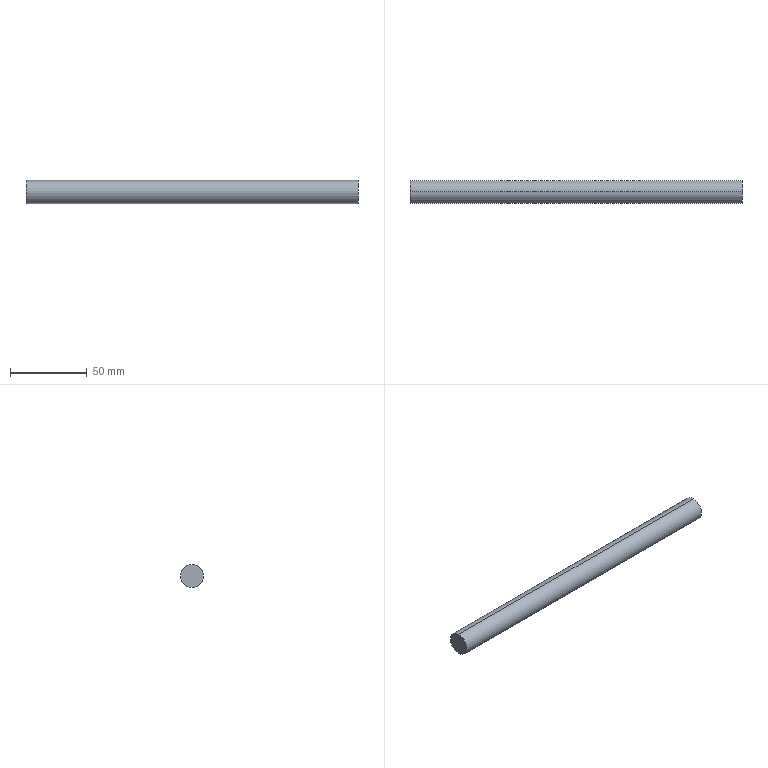Part | NX | features BREP 1 | 1 solid | 4 faces | box 216 x 15 x 15 mm | volume 38170 mm3 | cylinder 2 | plane 2 | commonest cylinder face diameters 15 x2
STEP:
#1=CARTESIAN_POINT('',(119.766,0.,7.5));
#2=VERTEX_POINT('',#1);
#3=CARTESIAN_POINT('',(119.766,0.,-7.5));
#4=VERTEX_POINT('',#3);
#5=CARTESIAN_POINT('',(119.766,0.,0.));
#6=DIRECTION('',(-1.,0.,0.));
#7=DIRECTION('',(0.,0.,1.));
#8=AXIS2_PLACEMENT_3D('',#5,#6,#7);
#9=CIRCLE('',#8,7.5);
#10=EDGE_CURVE('',#2,#4,#9,.T.);
#11=ORIENTED_EDGE('',*,*,#10,.T.);
#12=CARTESIAN_POINT('',(-96.234,0.,-7.5));
#13=VERTEX_POINT('',#12);
#14=CARTESIAN_POINT('',(-96.234,0.,-7.5));
#15=DIRECTION('',(-1.,0.,0.));
#16=VECTOR('',#15,1000.);
#17=LINE('',#14,#16);
#18=EDGE_CURVE('',#4,#13,#17,.T.);
#19=ORIENTED_EDGE('',*,*,#18,.T.);
#20=CARTESIAN_POINT('',(-96.234,0.,7.5));
#21=VERTEX_POINT('',#20);
#22=CARTESIAN_POINT('',(-96.234,0.,0.));
#23=DIRECTION('',(-1.,0.,0.));
#24=DIRECTION('',(0.,0.,1.));
#25=AXIS2_PLACEMENT_3D('',#22,#23,#24);
#26=CIRCLE('',#25,7.5);
#27=EDGE_CURVE('',#21,#13,#26,.T.);
#28=ORIENTED_EDGE('',*,*,#27,.F.);
#29=CARTESIAN_POINT('',(-96.234,0.,7.5));
#30=DIRECTION('',(-1.,0.,0.));
#31=VECTOR('',#30,1000.);
#32=LINE('',#29,#31);
#33=EDGE_CURVE('',#2,#21,#32,.T.);
#34=ORIENTED_EDGE('',*,*,#33,.F.);
#35=EDGE_LOOP('',(#11,#19,#28,#34));
#36=FACE_BOUND('',#35,.T.);
#37=CARTESIAN_POINT('',(-96.234,0.,0.));
#38=DIRECTION('',(-1.,0.,0.));
#39=DIRECTION('',(0.,0.,-1.));
#40=AXIS2_PLACEMENT_3D('',#37,#38,#39);
#41=CYLINDRICAL_SURFACE('',#40,7.5);
#42=ADVANCED_FACE('',(#36),#41,.T.);
#43=ORIENTED_EDGE('',*,*,#27,.T.);
#44=CARTESIAN_POINT('',(-96.234,0.,0.));
#45=DIRECTION('',(-1.,0.,0.));
#46=DIRECTION('',(0.,0.,1.));
#47=AXIS2_PLACEMENT_3D('',#44,#45,#46);
#48=CIRCLE('',#47,7.5);
#49=EDGE_CURVE('',#13,#21,#48,.T.);
#50=ORIENTED_EDGE('',*,*,#49,.T.);
#51=EDGE_LOOP('',(#43,#50));
#52=FACE_BOUND('',#51,.T.);
#53=CARTESIAN_POINT('',(-96.234,0.,0.));
#54=DIRECTION('',(1.,0.,0.));
#55=DIRECTION('',(0.,-1.,0.));
#56=AXIS2_PLACEMENT_3D('',#53,#54,#55);
#57=PLANE('',#56);
#58=ADVANCED_FACE('',(#52),#57,.F.);
#59=ORIENTED_EDGE('',*,*,#18,.F.);
#60=CARTESIAN_POINT('',(119.766,0.,0.));
#61=DIRECTION('',(-1.,0.,0.));
#62=DIRECTION('',(0.,0.,1.));
#63=AXIS2_PLACEMENT_3D('',#60,#61,#62);
#64=CIRCLE('',#63,7.5);
#65=EDGE_CURVE('',#4,#2,#64,.T.);
#66=ORIENTED_EDGE('',*,*,#65,.T.);
#67=ORIENTED_EDGE('',*,*,#33,.T.);
#68=ORIENTED_EDGE('',*,*,#49,.F.);
#69=EDGE_LOOP('',(#59,#66,#67,#68));
#70=FACE_BOUND('',#69,.T.);
#71=CARTESIAN_POINT('',(-96.234,0.,0.));
#72=DIRECTION('',(-1.,0.,0.));
#73=DIRECTION('',(0.,0.,-1.));
#74=AXIS2_PLACEMENT_3D('',#71,#72,#73);
#75=CYLINDRICAL_SURFACE('',#74,7.5);
#76=ADVANCED_FACE('',(#70),#75,.T.);
#77=ORIENTED_EDGE('',*,*,#10,.F.);
#78=ORIENTED_EDGE('',*,*,#65,.F.);
#79=EDGE_LOOP('',(#77,#78));
#80=FACE_BOUND('',#79,.T.);
#81=CARTESIAN_POINT('',(119.766,7.5,0.));
#82=DIRECTION('',(-1.,0.,0.));
#83=DIRECTION('',(0.,0.,-1.));
#84=AXIS2_PLACEMENT_3D('',#81,#82,#83);
#85=PLANE('',#84);
#86=ADVANCED_FACE('',(#80),#85,.F.);
#87=CLOSED_SHELL('',(#42,#58,#76,#86));
#88=MANIFOLD_SOLID_BREP('',#87);
#89=(LENGTH_UNIT()NAMED_UNIT(*)SI_UNIT(.MILLI.,.METRE.));
#90=UNCERTAINTY_MEASURE_WITH_UNIT(LENGTH_MEASURE(0.00001),#89,'','');
#91=(NAMED_UNIT(*)PLANE_ANGLE_UNIT()SI_UNIT($,.RADIAN.));
#92=(NAMED_UNIT(*)SI_UNIT($,.STERADIAN.)SOLID_ANGLE_UNIT());
#93=(GEOMETRIC_REPRESENTATION_CONTEXT(3)GLOBAL_UNCERTAINTY_ASSIGNED_CONTEXT((#90))GLOBAL_UNIT_ASSIGNED_CONTEXT((#89,#91,#92))REPRESENTATION_CONTEXT('',''));
#94=ADVANCED_BREP_SHAPE_REPRESENTATION('',(#88),#93);